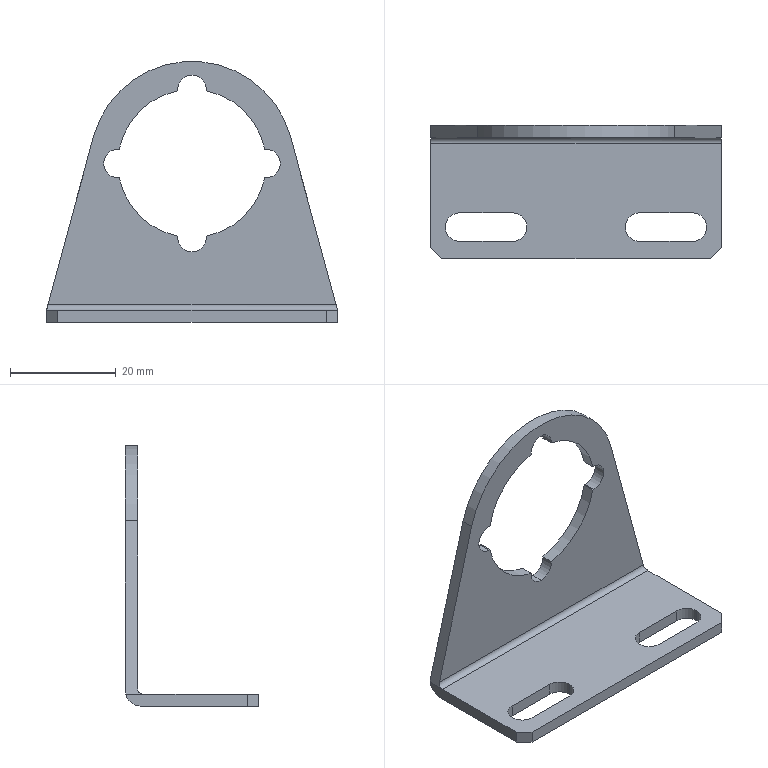Part | STEP file | AR20P-270AS(20)_BRACKET_HI | 1 solid | 37 faces | box 55 x 25.2 x 49.3 mm | volume 5580 mm3 | cylinder 22 | plane 15 | commonest cylinder face diameters 5.4 x15 28 x4 2 x1 6 x1 38.6 x1